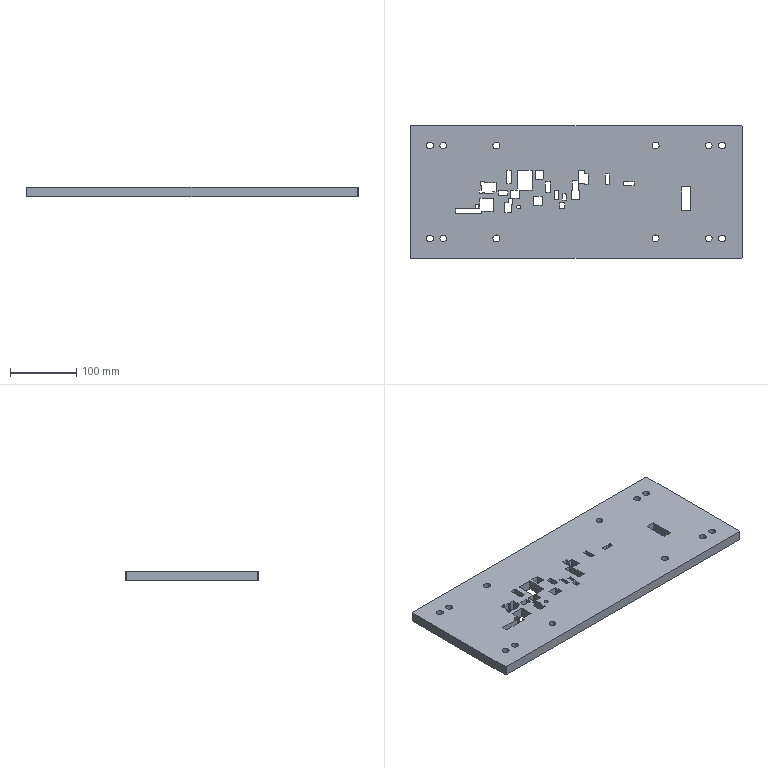Part | NX | features BREP 1 | 1 solid | 226 faces | box 500 x 200 x 15 mm | volume 1417253 mm3 | plane 120 | cylinder 106 | commonest cylinder face diameters 1 x92 10.5 x8 10.1 x4 6 x2